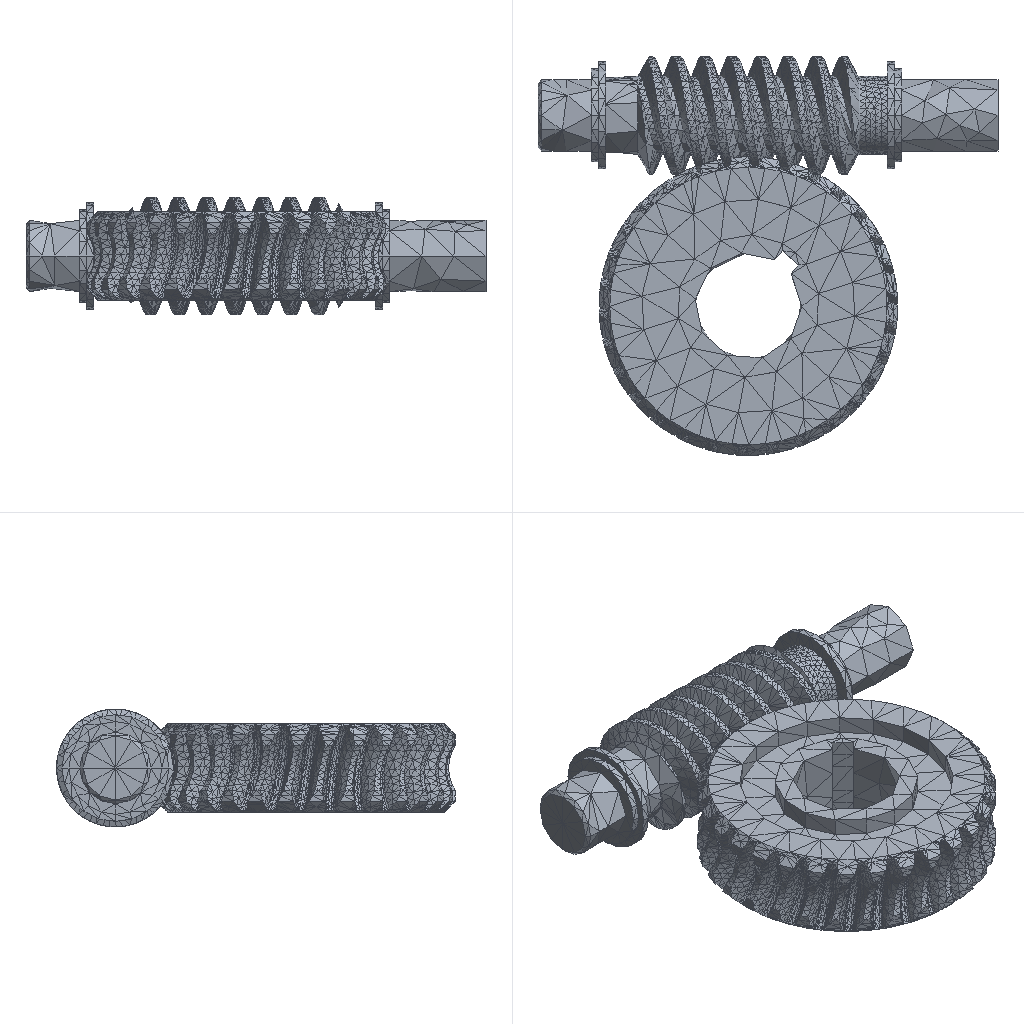Simulation study | ansys workbench
Set-up summary:
category,name,step,type,value,unit,region
solver,ansys_workbench
units,mm-N-s-tonne (MPa),,stated,"/units,MPA"
analysis,LS1,,static
load_step,LS1,LS1,static,nsubst=1; time=1
mesh,nodes,,,62755
mesh,elements,,,41547
element_type,SOLID187,,,35989
element_type,CONTA174,,,5242
element_type,TARGE170,,,316
material,45?,,E,200000,tonne s^-2 mm^-1
material,45?,,nu,0.3
material,45?,,density,7.85e-09,tonne mm^-3
material,45?,,conductivity,60.5,tonne mm s^-3 C^-1
material,45?,,specific_heat,4.34e+08,mm^2 s^-2 C^-1
material,45?,,cte,1.2e-05,C^-1
material,45?,,permeability,10000
material,45?,,resistivity,0.00017,ohm mm
material,Gray Cast Iron ht150,,E,75000,tonne s^-2 mm^-1
material,Gray Cast Iron ht150,,nu,0.25
material,Gray Cast Iron ht150,,density,7.2e-09,tonne mm^-3
material,Gray Cast Iron ht150,,cte,1.1e-05,C^-1
load,,LS1,moment,"180162 [dir=(0.9965, 0, 0.08304) n=6]",,all
bc,Fixed Supports,model,fixed,[dofs=ALL],,_FIXEDSU
contact,Contact Region,,bonded (always),element=CONTA174
contact,contact 2,,bonded (always),element=CONTA174
contact,contact 3,,bonded (always),element=CONTA174
named_set,______,,node,4010
named_set,______1,,node,8598
named_set,___1111,,node,13566
named_set,_FIXEDSU,,node,502
Ansys APDL input file, long lists of numbers shortened:
/batch
/config,noeldb,1     ! force off writing results to database
*get,_wallstrt,active,,time,wall
! ANSYS input file written by Workbench version 2022 R1
! File used for geometry attach:
/title,1111--____ (B5)
! ****** Begin Custom Load Command Snippet ******
/COM, ACT Extensions:
/COM,     LSDYNA, 2021.1
/COM,
! ****** End   Custom Load Command Snippet ******
*DIM,_wb_ProjectScratch_dir,string,248
_wb_ProjectScratch_dir(1) = ''
*DIM,_wb_SolverFiles_dir,string,248
_wb_SolverFiles_dir(1) = ''
*DIM,_wb_userfiles_dir,string,248
_wb_userfiles_dir(1) = ''
/com,--- Data in consistent NMM units. See Solving Units in the help system for more information.
/units,MPA
/nopr
/wb,file,start              !  signify a WB generated input file
/prep7
! Turn off shape checking because checks already performed inside WB mesher.
! See help system for more information.
SHPP,OFF,,NOWARN
/nolist
etcon,set             ! allow ANSYS to choose best KEYOP's for 180x elements, resets any applicable keyopt to MAPDL defaults
/com,*********** Nodes for the whole assembly ***********
nblock,3,,69028
(1i9,3e20.9e3)
        1    -4.400000000E+01     4.050000000E+01     3.900000000E-14
! (62752 more lines like these left out)
-1
/com,*********** Nodes for all Remote Points ***********
nblock,3
(1i9,3e20.9e3)
    62754    -2.462213175E+00     5.350000000E+01    -8.720013878E-10
    62755    -2.303291437E-01     4.365545299E-01     6.467840155E-02
-1
/wb,elem,start            !  set before creation of elements
/com,*********** Elements for Body 1 "Part1.2|_____" ***********
et,1,187
eblock,19,solid,,9035
(19i9)
        1        1        1        1        0        0        0        0       10        0        1     1582     2130     2705     2671    12447    14482    12451    12450
! (18069 more lines like these left out)
-1
/com,*********** Elements for Body 2 "11111111.3|_____" ***********
et,2,187
eblock,19,solid,,26954
(19i9)
        2        2        2        2        0        0        0        0       10        0     9036    19906    23681    21563    23665    46230    53963    46226    46229
! (53907 more lines like these left out)
-1
/wb,elem,end               !  done creating elements
/com,*********** Send User Defined Coordinate System(s) ***********
csys,0
toffst,273.15,  ! Temperature offset from absolute zero
/com,*********** Set Reference Temperature ***********
tref,22.
/wb,mat,start              !  starting to send materials
/com,*********** Send Materials ***********
Temperature = 'TEMP' ! Temperature
MP,DENS,1,7.85e-09,	! tonne mm^-3
MP,ALPX,1,1.2e-05,	! C^-1
MP,C,1,434000000,	! mm^2 s^-2 C^-1
MP,KXX,1,60.5,	! tonne mm s^-3 C^-1
MP,RSVX,1,0.00017,	! ohm mm
MP,EX,1,200000,	! tonne s^-2 mm^-1
MP,NUXY,1,0.3,
MP,MURX,1,10000,
MP,DENS,2,7.2e-09,	! tonne mm^-3
MP,ALPX,2,1.1e-05,	! C^-1
MP,EX,2,75000,	! tonne s^-2 mm^-1
MP,NUXY,2,0.25,
/wb,mat,end                !  done sending materials
!************************* Model Summary ********************
!Part1.2|_____,	45钢,	matid,	1
!11111111.3|_____,	灰铸铁ht150,	matid,	2
!************************* End Model Summary ********************
! get the diagonal of the bounding box. Needed later for other things
*get,_xmin,node,,mnloc,x
*get,_ymin,node,,mnloc,y
*get,_zmin,node,,mnloc,z
*get,_xmax,node,,mxloc,x
*get,_ymax,node,,mxloc,y
*get,_zmax,node,,mxloc,z
_ASMDIAG=(_xmax-_xmin)*(_xmax-_xmin)+(_ymax-_ymin)*(_ymax-_ymin)+(_zmax-_zmin)*(_zmax-_zmin)
_ASMDIAG=SQRT(_ASMDIAG)
/wb,contact,start          !  starting to send contact
/com,*********** Create Contact "接触区域" ***********
/com,            Real Constant Set For Above Contact Is 4 & 3
*set,tid,4
*set,cid,3
r,tid
r,cid
et,tid,170
et,cid,174
eblock,10,,,106
(15i9)
    49946        4        4        4        0      106      107     1359     1359     3566     3575     1359     3569
! (105 more lines like these left out)
-1
eblock,10,,,106
(15i9)
    50052        3        3        3        0      106      107     1359     1359     3566     3575     1359     3569
! (105 more lines like these left out)
-1
eblock,10,,,210
(15i9)
    50158        3        4        3        0    17574    17577    17575    17575    30760    30768    17575    30759
! (209 more lines like these left out)
-1
eblock,10,,,210
(15i9)
    50368        4        3        4        0    17574    17577    17575    17575    30760    30768    17575    30759
! (209 more lines like these left out)
-1
keyo,cid,8,2               ! auto create asymmetric contact (from Program Controlled setting)
keyo,cid,10,0              ! adjust contact stiffness each NR iteration (from Program Controlled setting)
keyo,cid,12,5              ! bonded always
keyo,cid,18,1              ! small sliding turned on by application
keyo,cid,2,0               ! augmented Lagrange (from Program Controlled setting)
keyo,cid,4,0               ! on Gauss point (from Program Controlled setting)
keyo,cid,9,1               ! ignore initial gaps/penetration
keyo,cid,7,0               ! No Prediction
rmod,tid,3,10.      ! FKN
rmod,tid,5,0.       ! ICONT
rmod,tid,6,0.       ! PINB
rmod,tid,10,0.      ! CNOF
rmod,tid,12,0.      ! FKT
rmod,tid,36,29      ! WB DSID
rmod,cid,3,10.      ! FKN
rmod,cid,5,0.       ! ICONT
rmod,cid,6,0.       ! PINB
rmod,cid,10,0.      ! CNOF
rmod,cid,12,0.      ! FKT
rmod,cid,36,29      ! WB DSID
nsel,all
esel,all
/wb,contact,end            !  done creating contacts
/com,*********** Send Named Selection as Node Component ***********
CMBLOCK,______  ,NODE,     4010
(8i10)
        19        20        21        22        23        24        25        26
! (501 more lines like these left out)
/com,*********** Send Named Selection as Node Component ***********
CMBLOCK,______1 ,NODE,     8598
(8i10)
       543       552       566       569       588       733       734       735
! (1074 more lines like these left out)
/com,*********** Send Named Selection as Node Component ***********
CMBLOCK,___1111 ,NODE,    13566
(8i10)
        29        31        36        37        38        47        48        49
! (1695 more lines like these left out)
/golist
/wb,load,start             !  starting to send loads
/com,*********** Fixed Supports ***********
CMBLOCK,_FIXEDSU,NODE,      502
(8i10)
        11        12        13        14        15        16        17        18
! (62 more lines like these left out)
cmsel,s,_FIXEDSU
d,all,all
nsel,all
/com,*********** Create Remote Point "内部远程点" ***********
! -------- Remote Point Used by "力矩" --------
*set,tid,6
*set,cid,5
et,cid,174
et,tid,170
keyo,tid,2,1               ! Don't fix the pilot node
keyo,tid,4,111111
keyo,cid,12,5              ! Bonded Contact
keyo,cid,4,1               ! Deformable RBE3 style load
keyo,cid,2,2               ! MPC style contact
eblock,10,,,1577
(15i9)
    50578        5        5        5        0       23     1333     1329     1329     2925    11368     1329     2924
! (1576 more lines like these left out)
-1
*set,_npilot,62754
_npilot42=_npilot
type,tid
mat ,cid
real,cid
tshape,pilo
en,52155,_npilot
tshape
/com,*********** Create Remote Point "内部远程点 2" ***********
! -------- Remote Point Used by "力矩 2" --------
*set,tid,8
*set,cid,7
et,cid,174
et,tid,170
keyo,tid,2,1               ! Don't fix the pilot node
keyo,tid,4,111111
keyo,cid,12,5              ! Bonded Contact
keyo,cid,4,1               ! Deformable RBE3 style load
keyo,cid,2,2               ! MPC style contact
eblock,10,,,3349
(15i9)
    52156        7        7        7        0      735     1166     1167     1167     7749    10522     1167     7750
! (3348 more lines like these left out)
-1
*set,_npilot,62755
_npilot48=_npilot
type,tid
mat ,cid
real,cid
tshape,pilo
en,55505,_npilot
tshape
/com,*********** Construct Moment Using Remote Attachment ***********
/com,*********** Construct Moment Using Remote Attachment ***********
/gst,on,on
fini
*get,_numnode,node,0,count
*get,_numelem,elem,0,count
*get, _MAXELEMNUM, elem, 0, NUM, MAX
*get, _MAXNODENUM, node, 0, NUM, MAX
*get, _MAXELEMTYPE, etyp, 0, NUM, MAX
*get, _MAXREALCONST, real, 0, NUM, MAX
/go
/wb,load,end               !  done creating loads
/com,--- Number of total nodes = %_numnode%
/com,--- Number of contact elements = 5558
/com,--- Number of spring elements = 0
/com,--- Number of bearing elements = 0
/com,--- Number of solid elements = 35989
/com,--- Number of condensed parts = 0
/com,--- Number of total elements = %_numelem%
*get,_wallbsol,active,,time,wall
/com,****************************************************************************
/com,*************************    SOLUTION       ********************************
/com,****************************************************************************
/solu
antype,0                   ! static analysis
_thickRatio=  1     ! Ratio of thick parts in the model
eqsl,pcg,1e-8,,,,,,1
cntr,print,1               ! print out contact info and also make no initial contact an error
dmpoption,emat,no             ! Don't combine emat file for DANSYS
dmpoption,esav,no             ! Don't combine esav file for DANSYS
nldiag,cont,iter           ! print out contact info each equilibrium iteration
rescontrol,,none                 ! Do not keep any restart files
/com,****************************************************
/com,******************* SOLVE FOR LS 1 OF 1 ****************
nsel,s,node,,62754
f,all,mx,179540.
f,all,my,0.
f,all,mz,0.
nsel,s,node,,62755
f,all,mx,0.
f,all,my,0.
f,all,mz,14960.
nsel,all
/nopr
/gopr
nsub,1,1,1
time,1.
outres,erase
outres,all,none
outres,nsol,all,
outres,rsol,all
outres,eangl,all
outres,etmp,all
outres,veng,all
outres,strs,all,
outres,epel,all,
outres,eppl,all,
outres,cont,all,
! *********** WB SOLVE COMMAND ***********
! check interactive state
*get,ANSINTER_,active,,int
*if,ANSINTER_,ne,0,then
/eof
*endif
solve
/com *************** Write FE CONNECTORS *********
CEWRITE,file,ce,,INTE
/com,****************************************************
/com,*************** FINISHED SOLVE FOR LS 1 *************
*get,_wallasol,active,,time,wall
/nopr
*get,_numnode,node,0,count
*get,_numelem,elem,0,count
*get, _MAXELEMNUM, elem, 0, NUM, MAX
*get, _MAXNODENUM, node, 0, NUM, MAX,,,INTERNAL
*get, _MAXELEMTYPE, etyp, 0, NUM, MAX
*get, _MAXREALCONST, real, 0, NUM, MAX
/gopr
*get,_PCGITER,active,,solu,cgiter
/post1
xmlo,ENCODING,ISO-8859-1
xmlo,parm
/xml,parm,xml
fini
/gopr
*get,_walldone,active,,time,wall
_preptime=(_wallbsol-_wallstrt)*3600
_solvtime=(_wallasol-_wallbsol)*3600
_posttime=(_walldone-_wallasol)*3600
_totaltim=(_walldone-_wallstrt)*3600
*get,_dlbratio,active,0,solu,dlbr
*get,_combtime,active,0,solu,comb
*get,_ssmode,active,0,solu,ssmm
*get,_ndofs,active,0,solu,ndof
*get,_sol_end_time,active,0,set,time
*if,_sol_end_time,eq,1.,then
/fclean				!clean distributed files
*endif
/com,--- Total number of nodes = %_numnode%
/com,--- Total number of elements = %_numelem%
/com,--- Element load balance ratio = %_dlbratio%
/com,--- Time to combine distributed files = %_combtime%
/com,--- Sparse memory mode = %_ssmode%
/com,--- Number of DOF = %_ndofs%
/wb,file,end               ! done with WB generated input
Results summary:
result,analyses[0].index,,,1
result,analyses[0].system,,,SYS
result,analyses[0].deck,,,deck.dat
result,analyses[0].solve_status,,,completed
result,analyses[0].analysis_type,,,static
result,analyses[0].physics,,,mechanical
result,analyses[0].unit_system,,,"NMM: mm, ton, N, s, mV, mA, degC"
result,analyses[0].n_sets,,,1
result,analyses[0].load_steps[0].set,set=1,,1
result,analyses[0].load_steps[0].time_or_freq,set=1,,1
result,analyses[0].load_steps[0].max_displacement_magnitude,set=1,,0.01471
result,analyses[0].load_steps[0].max_von_mises_nodal,set=1,,168.432
result,analyses[0].load_steps[0].reaction_force_sum_xyz[1],set=1,,1.22991e-05
result,analyses[0].load_steps[0].reaction_force_sum_xyz[2],set=1,,1.07193e-05
result,analyses[0].load_steps[0].reaction_force_sum_xyz[3],set=1,,2.84715e-07